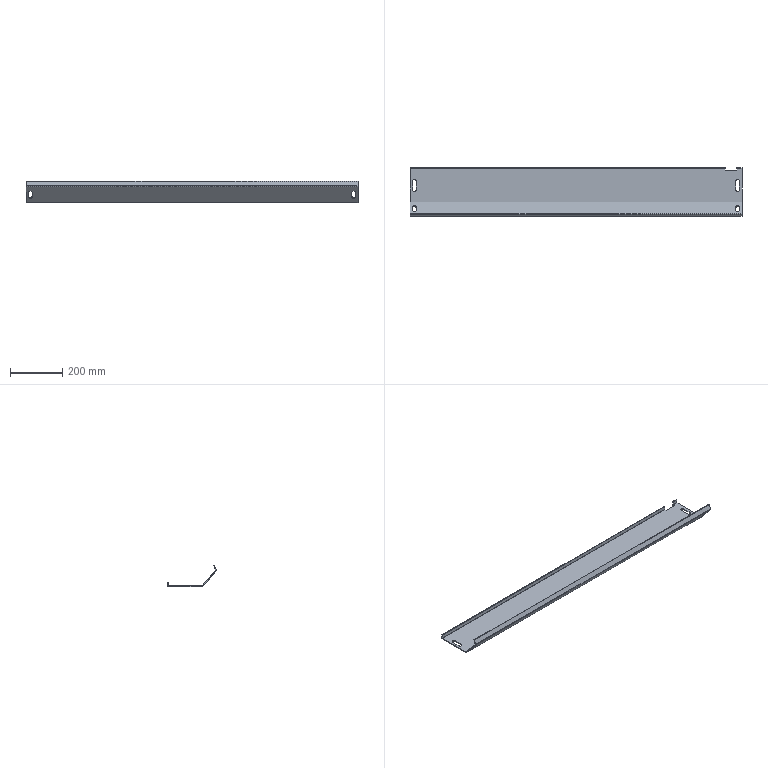Part | SolidWorks | features ICE 3, SM3dBend 3, Fillet 1, FlatPattern 1, SMBaseFlange 1, SheetMetal 1 | 1 solid | 62 faces | box 1270 x 184.784 x 82.347 mm | volume 924037 mm3 | plane 42 | cylinder 20 | commonest cylinder face diameters 13 x10 1.473 x4 7.473 x4 10 x2